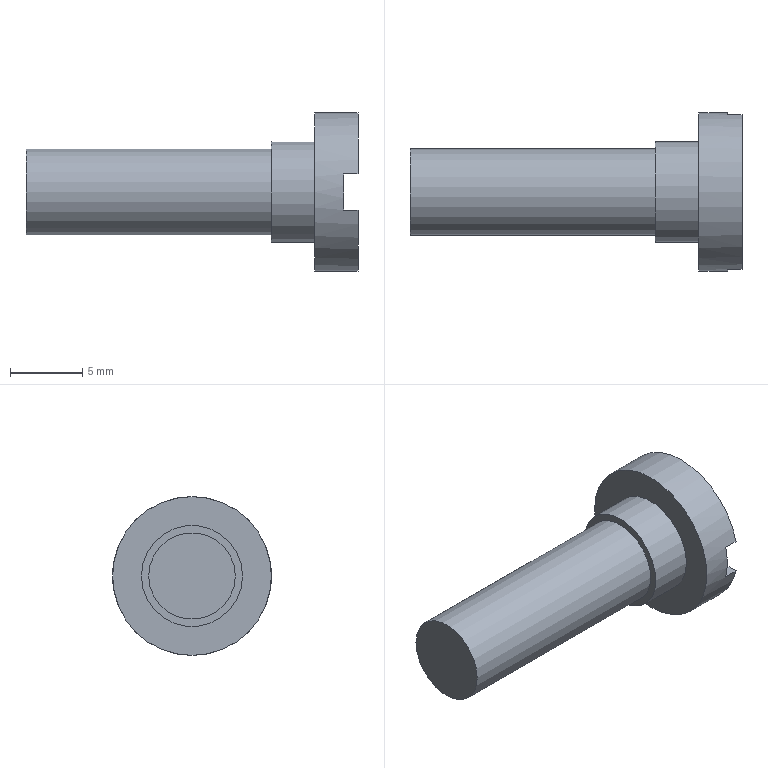Part | STEP file | 2-02.3 | 1 solid | 11 faces | box 23 x 11 x 11 mm | volume 853.955 mm3 | plane 8 | cylinder 3 | commonest cylinder face diameters 6 x1 7 x1 11 x1
STEP:
#1=CARTESIAN_POINT('',(0.,0.,0.));
#2=DIRECTION('',(0.,0.,1.));
#3=DIRECTION('',(1.,0.,0.));
#4=AXIS2_PLACEMENT_3D('',#1,#2,#3);
#5=CARTESIAN_POINT('',(0.,5.5,0.));
#6=VERTEX_POINT('',#5);
#7=CARTESIAN_POINT('',(0.,0.,0.));
#8=DIRECTION('',(1.,0.,0.));
#9=DIRECTION('',(0.,1.,0.));
#10=AXIS2_PLACEMENT_3D('',#7,#8,#9);
#11=CIRCLE('',#10,5.5);
#12=CARTESIAN_POINT('',(0.,-1.474,0.));
#13=DIRECTION('',(1.,0.,0.));
#14=DIRECTION('',(0.,0.,-1.));
#15=AXIS2_PLACEMENT_3D('',#12,#13,#14);
#16=PLANE('',#15);
#17=CARTESIAN_POINT('',(0.,1.474));
#18=DIRECTION('',(0.,1.));
#19=AXIS2_PLACEMENT_2D('',#17,#18);
#20=CIRCLE('',#19,5.5);
#21=(GEOMETRIC_REPRESENTATION_CONTEXT(2)PARAMETRIC_REPRESENTATION_CONTEXT()REPRESENTATION_CONTEXT('',''));
#22=DEFINITIONAL_REPRESENTATION('',(#20),#21);
#23=PCURVE('',#16,#22);
#24=CARTESIAN_POINT('',(0.,0.,0.));
#25=DIRECTION('',(1.,0.,0.));
#26=DIRECTION('',(0.,1.,0.));
#27=AXIS2_PLACEMENT_3D('',#24,#25,#26);
#28=CYLINDRICAL_SURFACE('',#27,5.5);
#29=CARTESIAN_POINT('',(0.,0.));
#30=DIRECTION('',(1.,0.));
#31=VECTOR('',#30,1.);
#32=LINE('',#29,#31);
#33=(GEOMETRIC_REPRESENTATION_CONTEXT(2)PARAMETRIC_REPRESENTATION_CONTEXT()REPRESENTATION_CONTEXT('',''));
#34=DEFINITIONAL_REPRESENTATION('',(#32),#33);
#35=PCURVE('',#28,#34);
#36=SURFACE_CURVE('',#11,(#23,#35),.PCURVE_S1.);
#37=EDGE_CURVE('',#6,#6,#36,.T.);
#38=ORIENTED_EDGE('',*,*,#37,.T.);
#39=EDGE_LOOP('',(#38));
#40=FACE_BOUND('',#39,.F.);
#41=CARTESIAN_POINT('',(0.,3.5,0.));
#42=VERTEX_POINT('',#41);
#43=CARTESIAN_POINT('',(0.,0.,0.));
#44=DIRECTION('',(1.,0.,0.));
#45=DIRECTION('',(0.,1.,0.));
#46=AXIS2_PLACEMENT_3D('',#43,#44,#45);
#47=CIRCLE('',#46,3.5);
#48=CARTESIAN_POINT('',(0.,1.474));
#49=DIRECTION('',(0.,1.));
#50=AXIS2_PLACEMENT_2D('',#48,#49);
#51=CIRCLE('',#50,3.5);
#52=(GEOMETRIC_REPRESENTATION_CONTEXT(2)PARAMETRIC_REPRESENTATION_CONTEXT()REPRESENTATION_CONTEXT('',''));
#53=DEFINITIONAL_REPRESENTATION('',(#51),#52);
#54=PCURVE('',#16,#53);
#55=CARTESIAN_POINT('',(0.,0.,0.));
#56=DIRECTION('',(-1.,0.,0.));
#57=DIRECTION('',(0.,1.,0.));
#58=AXIS2_PLACEMENT_3D('',#55,#56,#57);
#59=CYLINDRICAL_SURFACE('',#58,3.5);
#60=CARTESIAN_POINT('',(6.283,0.));
#61=DIRECTION('',(-1.,0.));
#62=VECTOR('',#61,1.);
#63=LINE('',#60,#62);
#64=(GEOMETRIC_REPRESENTATION_CONTEXT(2)PARAMETRIC_REPRESENTATION_CONTEXT()REPRESENTATION_CONTEXT('',''));
#65=DEFINITIONAL_REPRESENTATION('',(#63),#64);
#66=PCURVE('',#59,#65);
#67=SURFACE_CURVE('',#47,(#54,#66),.PCURVE_S1.);
#68=EDGE_CURVE('',#42,#42,#67,.T.);
#69=ORIENTED_EDGE('',*,*,#68,.F.);
#70=EDGE_LOOP('',(#69));
#71=FACE_BOUND('',#70,.F.);
#72=ADVANCED_FACE('',(#40,#71),#16,.F.);
#73=CARTESIAN_POINT('',(-3.,3.5,0.));
#74=VERTEX_POINT('',#73);
#75=CARTESIAN_POINT('',(0.,3.5,0.));
#76=DIRECTION('',(-1.,0.,0.));
#77=VECTOR('',#76,1.);
#78=LINE('',#75,#77);
#79=CARTESIAN_POINT('',(6.283,0.));
#80=DIRECTION('',(0.,1.));
#81=VECTOR('',#80,1.);
#82=LINE('',#79,#81);
#83=(GEOMETRIC_REPRESENTATION_CONTEXT(2)PARAMETRIC_REPRESENTATION_CONTEXT()REPRESENTATION_CONTEXT('',''));
#84=DEFINITIONAL_REPRESENTATION('',(#82),#83);
#85=PCURVE('',#59,#84);
#86=CARTESIAN_POINT('',(0.,0.));
#87=DIRECTION('',(0.,1.));
#88=VECTOR('',#87,1.);
#89=LINE('',#86,#88);
#90=(GEOMETRIC_REPRESENTATION_CONTEXT(2)PARAMETRIC_REPRESENTATION_CONTEXT()REPRESENTATION_CONTEXT('',''));
#91=DEFINITIONAL_REPRESENTATION('',(#89),#90);
#92=PCURVE('',#59,#91);
#93=SEAM_CURVE('',#78,(#85,#92),.PCURVE_S1.);
#94=EDGE_CURVE('',#42,#74,#93,.T.);
#95=ORIENTED_EDGE('',*,*,#94,.T.);
#96=CARTESIAN_POINT('',(-3.,0.,0.));
#97=DIRECTION('',(1.,0.,0.));
#98=DIRECTION('',(0.,1.,0.));
#99=AXIS2_PLACEMENT_3D('',#96,#97,#98);
#100=CIRCLE('',#99,3.5);
#101=CARTESIAN_POINT('',(6.283,3.));
#102=DIRECTION('',(-1.,0.));
#103=VECTOR('',#102,1.);
#104=LINE('',#101,#103);
#105=(GEOMETRIC_REPRESENTATION_CONTEXT(2)PARAMETRIC_REPRESENTATION_CONTEXT()REPRESENTATION_CONTEXT('',''));
#106=DEFINITIONAL_REPRESENTATION('',(#104),#105);
#107=PCURVE('',#59,#106);
#108=CARTESIAN_POINT('',(-3.,-0.9378,0.));
#109=DIRECTION('',(1.,0.,0.));
#110=DIRECTION('',(0.,0.,-1.));
#111=AXIS2_PLACEMENT_3D('',#108,#109,#110);
#112=PLANE('',#111);
#113=CARTESIAN_POINT('',(0.,0.9378));
#114=DIRECTION('',(0.,1.));
#115=AXIS2_PLACEMENT_2D('',#113,#114);
#116=CIRCLE('',#115,3.5);
#117=(GEOMETRIC_REPRESENTATION_CONTEXT(2)PARAMETRIC_REPRESENTATION_CONTEXT()REPRESENTATION_CONTEXT('',''));
#118=DEFINITIONAL_REPRESENTATION('',(#116),#117);
#119=PCURVE('',#112,#118);
#120=SURFACE_CURVE('',#100,(#107,#119),.PCURVE_S1.);
#121=EDGE_CURVE('',#74,#74,#120,.T.);
#122=ORIENTED_EDGE('',*,*,#121,.T.);
#123=ORIENTED_EDGE('',*,*,#94,.F.);
#124=ORIENTED_EDGE('',*,*,#68,.F.);
#125=EDGE_LOOP('',(#95,#122,#123,#124));
#126=FACE_BOUND('',#125,.T.);
#127=ADVANCED_FACE('',(#126),#59,.T.);
#128=ORIENTED_EDGE('',*,*,#121,.T.);
#129=EDGE_LOOP('',(#128));
#130=FACE_BOUND('',#129,.F.);
#131=CARTESIAN_POINT('',(-3.,3.,0.));
#132=VERTEX_POINT('',#131);
#133=CARTESIAN_POINT('',(-3.,0.,0.));
#134=DIRECTION('',(1.,0.,0.));
#135=DIRECTION('',(0.,1.,0.));
#136=AXIS2_PLACEMENT_3D('',#133,#134,#135);
#137=CIRCLE('',#136,3.);
#138=CARTESIAN_POINT('',(0.,0.9378));
#139=DIRECTION('',(0.,1.));
#140=AXIS2_PLACEMENT_2D('',#138,#139);
#141=CIRCLE('',#140,3.);
#142=(GEOMETRIC_REPRESENTATION_CONTEXT(2)PARAMETRIC_REPRESENTATION_CONTEXT()REPRESENTATION_CONTEXT('',''));
#143=DEFINITIONAL_REPRESENTATION('',(#141),#142);
#144=PCURVE('',#112,#143);
#145=CARTESIAN_POINT('',(-3.,0.,0.));
#146=DIRECTION('',(-1.,0.,0.));
#147=DIRECTION('',(0.,1.,0.));
#148=AXIS2_PLACEMENT_3D('',#145,#146,#147);
#149=CYLINDRICAL_SURFACE('',#148,3.);
#150=CARTESIAN_POINT('',(6.283,0.));
#151=DIRECTION('',(-1.,0.));
#152=VECTOR('',#151,1.);
#153=LINE('',#150,#152);
#154=(GEOMETRIC_REPRESENTATION_CONTEXT(2)PARAMETRIC_REPRESENTATION_CONTEXT()REPRESENTATION_CONTEXT('',''));
#155=DEFINITIONAL_REPRESENTATION('',(#153),#154);
#156=PCURVE('',#149,#155);
#157=SURFACE_CURVE('',#137,(#144,#156),.PCURVE_S1.);
#158=EDGE_CURVE('',#132,#132,#157,.T.);
#159=ORIENTED_EDGE('',*,*,#158,.F.);
#160=EDGE_LOOP('',(#159));
#161=FACE_BOUND('',#160,.F.);
#162=ADVANCED_FACE('',(#130,#161),#112,.F.);
#163=CARTESIAN_POINT('',(-20.,3.,0.));
#164=VERTEX_POINT('',#163);
#165=CARTESIAN_POINT('',(-3.,3.,0.));
#166=DIRECTION('',(-1.,0.,0.));
#167=VECTOR('',#166,1.);
#168=LINE('',#165,#167);
#169=CARTESIAN_POINT('',(6.283,0.));
#170=DIRECTION('',(0.,1.));
#171=VECTOR('',#170,1.);
#172=LINE('',#169,#171);
#173=(GEOMETRIC_REPRESENTATION_CONTEXT(2)PARAMETRIC_REPRESENTATION_CONTEXT()REPRESENTATION_CONTEXT('',''));
#174=DEFINITIONAL_REPRESENTATION('',(#172),#173);
#175=PCURVE('',#149,#174);
#176=CARTESIAN_POINT('',(0.,0.));
#177=DIRECTION('',(0.,1.));
#178=VECTOR('',#177,1.);
#179=LINE('',#176,#178);
#180=(GEOMETRIC_REPRESENTATION_CONTEXT(2)PARAMETRIC_REPRESENTATION_CONTEXT()REPRESENTATION_CONTEXT('',''));
#181=DEFINITIONAL_REPRESENTATION('',(#179),#180);
#182=PCURVE('',#149,#181);
#183=SEAM_CURVE('',#168,(#175,#182),.PCURVE_S1.);
#184=EDGE_CURVE('',#132,#164,#183,.T.);
#185=ORIENTED_EDGE('',*,*,#184,.T.);
#186=CARTESIAN_POINT('',(-20.,0.,0.));
#187=DIRECTION('',(1.,0.,0.));
#188=DIRECTION('',(0.,1.,0.));
#189=AXIS2_PLACEMENT_3D('',#186,#187,#188);
#190=CIRCLE('',#189,3.);
#191=CARTESIAN_POINT('',(6.283,17.));
#192=DIRECTION('',(-1.,0.));
#193=VECTOR('',#192,1.);
#194=LINE('',#191,#193);
#195=(GEOMETRIC_REPRESENTATION_CONTEXT(2)PARAMETRIC_REPRESENTATION_CONTEXT()REPRESENTATION_CONTEXT('',''));
#196=DEFINITIONAL_REPRESENTATION('',(#194),#195);
#197=PCURVE('',#149,#196);
#198=CARTESIAN_POINT('',(-20.,-0.8038,0.));
#199=DIRECTION('',(1.,0.,0.));
#200=DIRECTION('',(0.,0.,-1.));
#201=AXIS2_PLACEMENT_3D('',#198,#199,#200);
#202=PLANE('',#201);
#203=CARTESIAN_POINT('',(0.,0.8038));
#204=DIRECTION('',(0.,1.));
#205=AXIS2_PLACEMENT_2D('',#203,#204);
#206=CIRCLE('',#205,3.);
#207=(GEOMETRIC_REPRESENTATION_CONTEXT(2)PARAMETRIC_REPRESENTATION_CONTEXT()REPRESENTATION_CONTEXT('',''));
#208=DEFINITIONAL_REPRESENTATION('',(#206),#207);
#209=PCURVE('',#202,#208);
#210=SURFACE_CURVE('',#190,(#197,#209),.PCURVE_S1.);
#211=EDGE_CURVE('',#164,#164,#210,.T.);
#212=ORIENTED_EDGE('',*,*,#211,.T.);
#213=ORIENTED_EDGE('',*,*,#184,.F.);
#214=ORIENTED_EDGE('',*,*,#158,.F.);
#215=EDGE_LOOP('',(#185,#212,#213,#214));
#216=FACE_BOUND('',#215,.T.);
#217=ADVANCED_FACE('',(#216),#149,.T.);
#218=ORIENTED_EDGE('',*,*,#211,.T.);
#219=EDGE_LOOP('',(#218));
#220=FACE_BOUND('',#219,.F.);
#221=ADVANCED_FACE('',(#220),#202,.F.);
#222=CARTESIAN_POINT('',(3.,-5.356,-1.25));
#223=VERTEX_POINT('',#222);
#224=CARTESIAN_POINT('',(3.,5.356,-1.25));
#225=VERTEX_POINT('',#224);
#226=CARTESIAN_POINT('',(3.,0.,0.));
#227=DIRECTION('',(1.,0.,0.));
#228=DIRECTION('',(0.,-0.9738,-0.2273));
#229=AXIS2_PLACEMENT_3D('',#226,#227,#228);
#230=CIRCLE('',#229,5.5);
#231=CARTESIAN_POINT('',(3.,0.,0.));
#232=DIRECTION('',(1.,0.,0.));
#233=DIRECTION('',(0.,0.,-1.));
#234=AXIS2_PLACEMENT_3D('',#231,#232,#233);
#235=PLANE('',#234);
#236=CARTESIAN_POINT('',(0.,0.));
#237=DIRECTION('',(0.2273,-0.9738));
#238=AXIS2_PLACEMENT_2D('',#236,#237);
#239=CIRCLE('',#238,5.5);
#240=(GEOMETRIC_REPRESENTATION_CONTEXT(2)PARAMETRIC_REPRESENTATION_CONTEXT()REPRESENTATION_CONTEXT('',''));
#241=DEFINITIONAL_REPRESENTATION('',(#239),#240);
#242=PCURVE('',#235,#241);
#243=CARTESIAN_POINT('',(3.371,3.));
#244=DIRECTION('',(1.,0.));
#245=VECTOR('',#244,1.);
#246=LINE('',#243,#245);
#247=(GEOMETRIC_REPRESENTATION_CONTEXT(2)PARAMETRIC_REPRESENTATION_CONTEXT()REPRESENTATION_CONTEXT('',''));
#248=DEFINITIONAL_REPRESENTATION('',(#246),#247);
#249=PCURVE('',#28,#248);
#250=SURFACE_CURVE('',#230,(#242,#249),.PCURVE_S1.);
#251=EDGE_CURVE('',#223,#225,#250,.T.);
#252=ORIENTED_EDGE('',*,*,#251,.T.);
#253=CARTESIAN_POINT('',(3.,-5.356,-1.25));
#254=DIRECTION('',(0.,1.,0.));
#255=VECTOR('',#254,1.);
#256=LINE('',#253,#255);
#257=CARTESIAN_POINT('',(1.25,-5.356));
#258=DIRECTION('',(0.,1.));
#259=VECTOR('',#258,1.);
#260=LINE('',#257,#259);
#261=(GEOMETRIC_REPRESENTATION_CONTEXT(2)PARAMETRIC_REPRESENTATION_CONTEXT()REPRESENTATION_CONTEXT('',''));
#262=DEFINITIONAL_REPRESENTATION('',(#260),#261);
#263=PCURVE('',#235,#262);
#264=CARTESIAN_POINT('',(3.,0.,-1.25));
#265=DIRECTION('',(0.,0.,1.));
#266=DIRECTION('',(1.,0.,0.));
#267=AXIS2_PLACEMENT_3D('',#264,#265,#266);
#268=PLANE('',#267);
#269=CARTESIAN_POINT('',(0.,-5.356));
#270=DIRECTION('',(0.,1.));
#271=VECTOR('',#270,1.);
#272=LINE('',#269,#271);
#273=(GEOMETRIC_REPRESENTATION_CONTEXT(2)PARAMETRIC_REPRESENTATION_CONTEXT()REPRESENTATION_CONTEXT('',''));
#274=DEFINITIONAL_REPRESENTATION('',(#272),#273);
#275=PCURVE('',#268,#274);
#276=SURFACE_CURVE('',#256,(#263,#275),.PCURVE_S1.);
#277=EDGE_CURVE('',#223,#225,#276,.T.);
#278=ORIENTED_EDGE('',*,*,#277,.F.);
#279=EDGE_LOOP('',(#252,#278));
#280=FACE_BOUND('',#279,.T.);
#281=ADVANCED_FACE('',(#280),#235,.T.);
#282=CARTESIAN_POINT('',(3.,5.356,1.25));
#283=VERTEX_POINT('',#282);
#284=CARTESIAN_POINT('',(3.,-5.356,1.25));
#285=VERTEX_POINT('',#284);
#286=CARTESIAN_POINT('',(3.,0.,0.));
#287=DIRECTION('',(1.,0.,0.));
#288=DIRECTION('',(0.,0.9738,0.2273));
#289=AXIS2_PLACEMENT_3D('',#286,#287,#288);
#290=CIRCLE('',#289,5.5);
#291=CARTESIAN_POINT('',(3.,0.,0.));
#292=DIRECTION('',(1.,0.,0.));
#293=DIRECTION('',(0.,0.,-1.));
#294=AXIS2_PLACEMENT_3D('',#291,#292,#293);
#295=PLANE('',#294);
#296=CARTESIAN_POINT('',(0.,0.));
#297=DIRECTION('',(-0.2273,0.9738));
#298=AXIS2_PLACEMENT_2D('',#296,#297);
#299=CIRCLE('',#298,5.5);
#300=(GEOMETRIC_REPRESENTATION_CONTEXT(2)PARAMETRIC_REPRESENTATION_CONTEXT()REPRESENTATION_CONTEXT('',''));
#301=DEFINITIONAL_REPRESENTATION('',(#299),#300);
#302=PCURVE('',#295,#301);
#303=CARTESIAN_POINT('',(0.2293,3.));
#304=DIRECTION('',(1.,0.));
#305=VECTOR('',#304,1.);
#306=LINE('',#303,#305);
#307=(GEOMETRIC_REPRESENTATION_CONTEXT(2)PARAMETRIC_REPRESENTATION_CONTEXT()REPRESENTATION_CONTEXT('',''));
#308=DEFINITIONAL_REPRESENTATION('',(#306),#307);
#309=PCURVE('',#28,#308);
#310=SURFACE_CURVE('',#290,(#302,#309),.PCURVE_S1.);
#311=EDGE_CURVE('',#283,#285,#310,.T.);
#312=ORIENTED_EDGE('',*,*,#311,.T.);
#313=CARTESIAN_POINT('',(3.,5.356,1.25));
#314=DIRECTION('',(0.,-1.,0.));
#315=VECTOR('',#314,1.);
#316=LINE('',#313,#315);
#317=CARTESIAN_POINT('',(-1.25,5.356));
#318=DIRECTION('',(0.,-1.));
#319=VECTOR('',#318,1.);
#320=LINE('',#317,#319);
#321=(GEOMETRIC_REPRESENTATION_CONTEXT(2)PARAMETRIC_REPRESENTATION_CONTEXT()REPRESENTATION_CONTEXT('',''));
#322=DEFINITIONAL_REPRESENTATION('',(#320),#321);
#323=PCURVE('',#295,#322);
#324=CARTESIAN_POINT('',(3.,0.,1.25));
#325=DIRECTION('',(0.,0.,-1.));
#326=DIRECTION('',(-1.,0.,0.));
#327=AXIS2_PLACEMENT_3D('',#324,#325,#326);
#328=PLANE('',#327);
#329=CARTESIAN_POINT('',(0.,5.356));
#330=DIRECTION('',(0.,-1.));
#331=VECTOR('',#330,1.);
#332=LINE('',#329,#331);
#333=(GEOMETRIC_REPRESENTATION_CONTEXT(2)PARAMETRIC_REPRESENTATION_CONTEXT()REPRESENTATION_CONTEXT('',''));
#334=DEFINITIONAL_REPRESENTATION('',(#332),#333);
#335=PCURVE('',#328,#334);
#336=SURFACE_CURVE('',#316,(#323,#335),.PCURVE_S1.);
#337=EDGE_CURVE('',#283,#285,#336,.T.);
#338=ORIENTED_EDGE('',*,*,#337,.F.);
#339=EDGE_LOOP('',(#312,#338));
#340=FACE_BOUND('',#339,.T.);
#341=ADVANCED_FACE('',(#340),#295,.T.);
#342=ORIENTED_EDGE('',*,*,#37,.T.);
#343=CARTESIAN_POINT('',(2.,5.5,0.));
#344=VERTEX_POINT('',#343);
#345=CARTESIAN_POINT('',(0.,5.5,0.));
#346=DIRECTION('',(1.,0.,0.));
#347=VECTOR('',#346,1.);
#348=LINE('',#345,#347);
#349=CARTESIAN_POINT('',(6.283,0.));
#350=DIRECTION('',(0.,1.));
#351=VECTOR('',#350,1.);
#352=LINE('',#349,#351);
#353=(GEOMETRIC_REPRESENTATION_CONTEXT(2)PARAMETRIC_REPRESENTATION_CONTEXT()REPRESENTATION_CONTEXT('',''));
#354=DEFINITIONAL_REPRESENTATION('',(#352),#353);
#355=PCURVE('',#28,#354);
#356=CARTESIAN_POINT('',(0.,0.));
#357=DIRECTION('',(0.,1.));
#358=VECTOR('',#357,1.);
#359=LINE('',#356,#358);
#360=(GEOMETRIC_REPRESENTATION_CONTEXT(2)PARAMETRIC_REPRESENTATION_CONTEXT()REPRESENTATION_CONTEXT('',''));
#361=DEFINITIONAL_REPRESENTATION('',(#359),#360);
#362=PCURVE('',#28,#361);
#363=SEAM_CURVE('',#348,(#355,#362),.PCURVE_S1.);
#364=EDGE_CURVE('',#6,#344,#363,.T.);
#365=ORIENTED_EDGE('',*,*,#364,.T.);
#366=CARTESIAN_POINT('',(2.,5.356,-1.25));
#367=VERTEX_POINT('',#366);
#368=CARTESIAN_POINT('',(2.,0.,0.));
#369=DIRECTION('',(1.,0.,0.));
#370=DIRECTION('',(0.,0.9738,-0.2273));
#371=AXIS2_PLACEMENT_3D('',#368,#369,#370);
#372=CIRCLE('',#371,5.5);
#373=CARTESIAN_POINT('',(6.054,2.));
#374=DIRECTION('',(1.,0.));
#375=VECTOR('',#374,1.);
#376=LINE('',#373,#375);
#377=(GEOMETRIC_REPRESENTATION_CONTEXT(2)PARAMETRIC_REPRESENTATION_CONTEXT()REPRESENTATION_CONTEXT('',''));
#378=DEFINITIONAL_REPRESENTATION('',(#376),#377);
#379=PCURVE('',#28,#378);
#380=CARTESIAN_POINT('',(2.,0.,0.));
#381=DIRECTION('',(1.,0.,0.));
#382=DIRECTION('',(0.,0.,-1.));
#383=AXIS2_PLACEMENT_3D('',#380,#381,#382);
#384=PLANE('',#383);
#385=CARTESIAN_POINT('',(0.,0.));
#386=DIRECTION('',(0.2273,0.9738));
#387=AXIS2_PLACEMENT_2D('',#385,#386);
#388=CIRCLE('',#387,5.5);
#389=(GEOMETRIC_REPRESENTATION_CONTEXT(2)PARAMETRIC_REPRESENTATION_CONTEXT()REPRESENTATION_CONTEXT('',''));
#390=DEFINITIONAL_REPRESENTATION('',(#388),#389);
#391=PCURVE('',#384,#390);
#392=SURFACE_CURVE('',#372,(#379,#391),.PCURVE_S1.);
#393=EDGE_CURVE('',#367,#344,#392,.T.);
#394=ORIENTED_EDGE('',*,*,#393,.F.);
#395=CARTESIAN_POINT('',(3.,5.356,-1.25));
#396=DIRECTION('',(-1.,0.,0.));
#397=VECTOR('',#396,1.);
#398=LINE('',#395,#397);
#399=CARTESIAN_POINT('',(6.054,3.));
#400=DIRECTION('',(0.,-1.));
#401=VECTOR('',#400,1.);
#402=LINE('',#399,#401);
#403=(GEOMETRIC_REPRESENTATION_CONTEXT(2)PARAMETRIC_REPRESENTATION_CONTEXT()REPRESENTATION_CONTEXT('',''));
#404=DEFINITIONAL_REPRESENTATION('',(#402),#403);
#405=PCURVE('',#28,#404);
#406=CARTESIAN_POINT('',(0.,5.356));
#407=DIRECTION('',(-1.,0.));
#408=VECTOR('',#407,1.);
#409=LINE('',#406,#408);
#410=(GEOMETRIC_REPRESENTATION_CONTEXT(2)PARAMETRIC_REPRESENTATION_CONTEXT()REPRESENTATION_CONTEXT('',''));
#411=DEFINITIONAL_REPRESENTATION('',(#409),#410);
#412=PCURVE('',#268,#411);
#413=SURFACE_CURVE('',#398,(#405,#412),.PCURVE_S1.);
#414=EDGE_CURVE('',#225,#367,#413,.T.);
#415=ORIENTED_EDGE('',*,*,#414,.F.);
#416=ORIENTED_EDGE('',*,*,#251,.F.);
#417=CARTESIAN_POINT('',(2.,-5.356,-1.25));
#418=VERTEX_POINT('',#417);
#419=CARTESIAN_POINT('',(2.,-5.356,-1.25));
#420=DIRECTION('',(1.,0.,0.));
#421=VECTOR('',#420,1.);
#422=LINE('',#419,#421);
#423=CARTESIAN_POINT('',(3.371,2.));
#424=DIRECTION('',(0.,1.));
#425=VECTOR('',#424,1.);
#426=LINE('',#423,#425);
#427=(GEOMETRIC_REPRESENTATION_CONTEXT(2)PARAMETRIC_REPRESENTATION_CONTEXT()REPRESENTATION_CONTEXT('',''));
#428=DEFINITIONAL_REPRESENTATION('',(#426),#427);
#429=PCURVE('',#28,#428);
#430=CARTESIAN_POINT('',(-1.,-5.356));
#431=DIRECTION('',(1.,0.));
#432=VECTOR('',#431,1.);
#433=LINE('',#430,#432);
#434=(GEOMETRIC_REPRESENTATION_CONTEXT(2)PARAMETRIC_REPRESENTATION_CONTEXT()REPRESENTATION_CONTEXT('',''));
#435=DEFINITIONAL_REPRESENTATION('',(#433),#434);
#436=PCURVE('',#268,#435);
#437=SURFACE_CURVE('',#422,(#429,#436),.PCURVE_S1.);
#438=EDGE_CURVE('',#418,#223,#437,.T.);
#439=ORIENTED_EDGE('',*,*,#438,.F.);
#440=CARTESIAN_POINT('',(2.,-5.356,1.25));
#441=VERTEX_POINT('',#440);
#442=CARTESIAN_POINT('',(2.,0.,0.));
#443=DIRECTION('',(1.,0.,0.));
#444=DIRECTION('',(0.,-0.9738,0.2273));
#445=AXIS2_PLACEMENT_3D('',#442,#443,#444);
#446=CIRCLE('',#445,5.5);
#447=CARTESIAN_POINT('',(2.912,2.));
#448=DIRECTION('',(1.,0.));
#449=VECTOR('',#448,1.);
#450=LINE('',#447,#449);
#451=(GEOMETRIC_REPRESENTATION_CONTEXT(2)PARAMETRIC_REPRESENTATION_CONTEXT()REPRESENTATION_CONTEXT('',''));
#452=DEFINITIONAL_REPRESENTATION('',(#450),#451);
#453=PCURVE('',#28,#452);
#454=CARTESIAN_POINT('',(0.,0.));
#455=DIRECTION('',(-0.2273,-0.9738));
#456=AXIS2_PLACEMENT_2D('',#454,#455);
#457=CIRCLE('',#456,5.5);
#458=(GEOMETRIC_REPRESENTATION_CONTEXT(2)PARAMETRIC_REPRESENTATION_CONTEXT()REPRESENTATION_CONTEXT('',''));
#459=DEFINITIONAL_REPRESENTATION('',(#457),#458);
#460=PCURVE('',#384,#459);
#461=SURFACE_CURVE('',#446,(#453,#460),.PCURVE_S1.);
#462=EDGE_CURVE('',#441,#418,#461,.T.);
#463=ORIENTED_EDGE('',*,*,#462,.F.);
#464=CARTESIAN_POINT('',(3.,-5.356,1.25));
#465=DIRECTION('',(-1.,0.,0.));
#466=VECTOR('',#465,1.);
#467=LINE('',#464,#466);
#468=CARTESIAN_POINT('',(2.912,3.));
#469=DIRECTION('',(0.,-1.));
#470=VECTOR('',#469,1.);
#471=LINE('',#468,#470);
#472=(GEOMETRIC_REPRESENTATION_CONTEXT(2)PARAMETRIC_REPRESENTATION_CONTEXT()REPRESENTATION_CONTEXT('',''));
#473=DEFINITIONAL_REPRESENTATION('',(#471),#472);
#474=PCURVE('',#28,#473);
#475=CARTESIAN_POINT('',(0.,-5.356));
#476=DIRECTION('',(1.,0.));
#477=VECTOR('',#476,1.);
#478=LINE('',#475,#477);
#479=(GEOMETRIC_REPRESENTATION_CONTEXT(2)PARAMETRIC_REPRESENTATION_CONTEXT()REPRESENTATION_CONTEXT('',''));
#480=DEFINITIONAL_REPRESENTATION('',(#478),#479);
#481=PCURVE('',#328,#480);
#482=SURFACE_CURVE('',#467,(#474,#481),.PCURVE_S1.);
#483=EDGE_CURVE('',#285,#441,#482,.T.);
#484=ORIENTED_EDGE('',*,*,#483,.F.);
#485=ORIENTED_EDGE('',*,*,#311,.F.);
#486=CARTESIAN_POINT('',(2.,5.356,1.25));
#487=VERTEX_POINT('',#486);
#488=CARTESIAN_POINT('',(2.,5.356,1.25));
#489=DIRECTION('',(1.,0.,0.));
#490=VECTOR('',#489,1.);
#491=LINE('',#488,#490);
#492=CARTESIAN_POINT('',(0.2293,2.));
#493=DIRECTION('',(0.,1.));
#494=VECTOR('',#493,1.);
#495=LINE('',#492,#494);
#496=(GEOMETRIC_REPRESENTATION_CONTEXT(2)PARAMETRIC_REPRESENTATION_CONTEXT()REPRESENTATION_CONTEXT('',''));
#497=DEFINITIONAL_REPRESENTATION('',(#495),#496);
#498=PCURVE('',#28,#497);
#499=CARTESIAN_POINT('',(1.,5.356));
#500=DIRECTION('',(-1.,0.));
#501=VECTOR('',#500,1.);
#502=LINE('',#499,#501);
#503=(GEOMETRIC_REPRESENTATION_CONTEXT(2)PARAMETRIC_REPRESENTATION_CONTEXT()REPRESENTATION_CONTEXT('',''));
#504=DEFINITIONAL_REPRESENTATION('',(#502),#503);
#505=PCURVE('',#328,#504);
#506=SURFACE_CURVE('',#491,(#498,#505),.PCURVE_S1.);
#507=EDGE_CURVE('',#487,#283,#506,.T.);
#508=ORIENTED_EDGE('',*,*,#507,.F.);
#509=CARTESIAN_POINT('',(2.,0.,0.));
#510=DIRECTION('',(1.,0.,0.));
#511=DIRECTION('',(0.,1.,0.));
#512=AXIS2_PLACEMENT_3D('',#509,#510,#511);
#513=CIRCLE('',#512,5.5);
#514=CARTESIAN_POINT('',(0.,2.));
#515=DIRECTION('',(1.,0.));
#516=VECTOR('',#515,1.);
#517=LINE('',#514,#516);
#518=(GEOMETRIC_REPRESENTATION_CONTEXT(2)PARAMETRIC_REPRESENTATION_CONTEXT()REPRESENTATION_CONTEXT('',''));
#519=DEFINITIONAL_REPRESENTATION('',(#517),#518);
#520=PCURVE('',#28,#519);
#521=CARTESIAN_POINT('',(0.,0.));
#522=DIRECTION('',(0.,1.));
#523=AXIS2_PLACEMENT_2D('',#521,#522);
#524=CIRCLE('',#523,5.5);
#525=(GEOMETRIC_REPRESENTATION_CONTEXT(2)PARAMETRIC_REPRESENTATION_CONTEXT()REPRESENTATION_CONTEXT('',''));
#526=DEFINITIONAL_REPRESENTATION('',(#524),#525);
#527=PCURVE('',#384,#526);
#528=SURFACE_CURVE('',#513,(#520,#527),.PCURVE_S1.);
#529=EDGE_CURVE('',#344,#487,#528,.T.);
#530=ORIENTED_EDGE('',*,*,#529,.F.);
#531=ORIENTED_EDGE('',*,*,#364,.F.);
#532=EDGE_LOOP('',(#342,#365,#394,#415,#416,#439,#463,#484,#485,#508,#530,#531));
#533=FACE_BOUND('',#532,.T.);
#534=ADVANCED_FACE('',(#533),#28,.T.);
#535=CARTESIAN_POINT('',(2.,-5.356,1.25));
#536=DIRECTION('',(0.,1.,0.));
#537=VECTOR('',#536,1.);
#538=LINE('',#535,#537);
#539=CARTESIAN_POINT('',(-1.25,-5.356));
#540=DIRECTION('',(0.,1.));
#541=VECTOR('',#540,1.);
#542=LINE('',#539,#541);
#543=(GEOMETRIC_REPRESENTATION_CONTEXT(2)PARAMETRIC_REPRESENTATION_CONTEXT()REPRESENTATION_CONTEXT('',''));
#544=DEFINITIONAL_REPRESENTATION('',(#542),#543);
#545=PCURVE('',#384,#544);
#546=CARTESIAN_POINT('',(1.,-5.356));
#547=DIRECTION('',(0.,1.));
#548=VECTOR('',#547,1.);
#549=LINE('',#546,#548);
#550=(GEOMETRIC_REPRESENTATION_CONTEXT(2)PARAMETRIC_REPRESENTATION_CONTEXT()REPRESENTATION_CONTEXT('',''));
#551=DEFINITIONAL_REPRESENTATION('',(#549),#550);
#552=PCURVE('',#328,#551);
#553=SURFACE_CURVE('',#538,(#545,#552),.PCURVE_S1.);
#554=EDGE_CURVE('',#441,#487,#553,.T.);
#555=ORIENTED_EDGE('',*,*,#554,.F.);
#556=ORIENTED_EDGE('',*,*,#462,.T.);
#557=CARTESIAN_POINT('',(2.,-5.356,-1.25));
#558=DIRECTION('',(0.,1.,0.));
#559=VECTOR('',#558,1.);
#560=LINE('',#557,#559);
#561=CARTESIAN_POINT('',(1.25,-5.356));
#562=DIRECTION('',(0.,1.));
#563=VECTOR('',#562,1.);
#564=LINE('',#561,#563);
#565=(GEOMETRIC_REPRESENTATION_CONTEXT(2)PARAMETRIC_REPRESENTATION_CONTEXT()REPRESENTATION_CONTEXT('',''));
#566=DEFINITIONAL_REPRESENTATION('',(#564),#565);
#567=PCURVE('',#384,#566);
#568=CARTESIAN_POINT('',(-1.,-5.356));
#569=DIRECTION('',(0.,1.));
#570=VECTOR('',#569,1.);
#571=LINE('',#568,#570);
#572=(GEOMETRIC_REPRESENTATION_CONTEXT(2)PARAMETRIC_REPRESENTATION_CONTEXT()REPRESENTATION_CONTEXT('',''));
#573=DEFINITIONAL_REPRESENTATION('',(#571),#572);
#574=PCURVE('',#268,#573);
#575=SURFACE_CURVE('',#560,(#567,#574),.PCURVE_S1.);
#576=EDGE_CURVE('',#418,#367,#575,.T.);
#577=ORIENTED_EDGE('',*,*,#576,.T.);
#578=ORIENTED_EDGE('',*,*,#393,.T.);
#579=ORIENTED_EDGE('',*,*,#529,.T.);
#580=EDGE_LOOP('',(#555,#556,#577,#578,#579));
#581=FACE_BOUND('',#580,.T.);
#582=ADVANCED_FACE('',(#581),#384,.T.);
#583=ORIENTED_EDGE('',*,*,#576,.F.);
#584=ORIENTED_EDGE('',*,*,#438,.T.);
#585=ORIENTED_EDGE('',*,*,#277,.T.);
#586=ORIENTED_EDGE('',*,*,#414,.T.);
#587=EDGE_LOOP('',(#583,#584,#585,#586));
#588=FACE_BOUND('',#587,.T.);
#589=ADVANCED_FACE('',(#588),#268,.T.);
#590=ORIENTED_EDGE('',*,*,#554,.T.);
#591=ORIENTED_EDGE('',*,*,#507,.T.);
#592=ORIENTED_EDGE('',*,*,#337,.T.);
#593=ORIENTED_EDGE('',*,*,#483,.T.);
#594=EDGE_LOOP('',(#590,#591,#592,#593));
#595=FACE_BOUND('',#594,.T.);
#596=ADVANCED_FACE('',(#595),#328,.T.);
#597=CLOSED_SHELL('',(#72,#127,#162,#217,#221,#281,#341,#534,#582,#589,#596));
#598=MANIFOLD_SOLID_BREP('',#597);
#599=(LENGTH_UNIT()NAMED_UNIT(*)SI_UNIT(.MILLI.,.METRE.));
#600=UNCERTAINTY_MEASURE_WITH_UNIT(LENGTH_MEASURE(0.0000001),#599,'','');
#601=(NAMED_UNIT(*)PLANE_ANGLE_UNIT()SI_UNIT($,.RADIAN.));
#602=(NAMED_UNIT(*)SI_UNIT($,.STERADIAN.)SOLID_ANGLE_UNIT());
#603=(GEOMETRIC_REPRESENTATION_CONTEXT(3)GLOBAL_UNCERTAINTY_ASSIGNED_CONTEXT((#600))GLOBAL_UNIT_ASSIGNED_CONTEXT((#599,#601,#602))REPRESENTATION_CONTEXT('',''));
#604=ADVANCED_BREP_SHAPE_REPRESENTATION('',(#4,#598),#603);